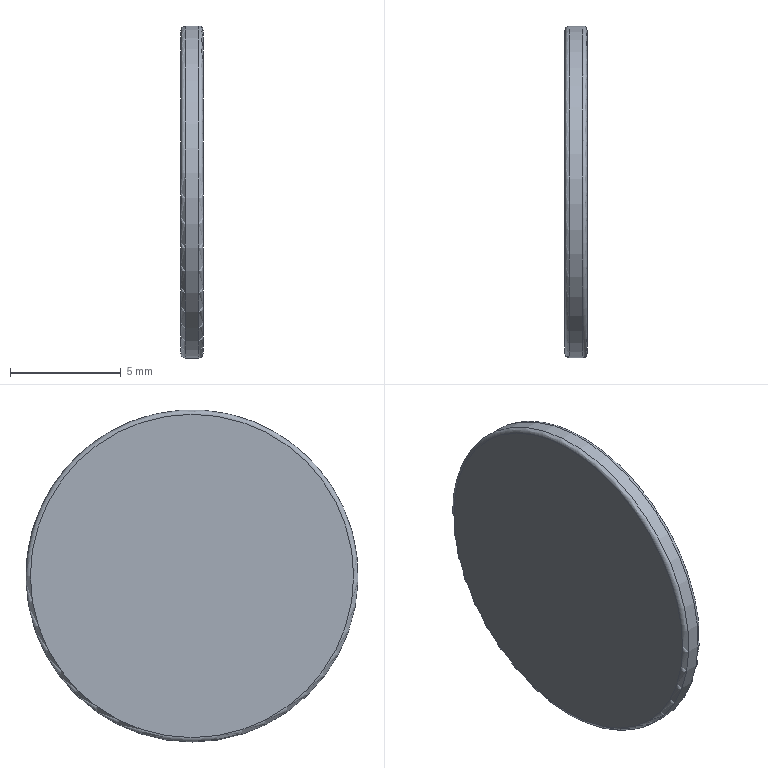Part | STEP file | Tube necking machine_id234_x_t | 1 solid | 5 faces | box 1 x 15 x 15 mm | volume 175.91 mm3 | plane 2 | torus 2 | cylinder 1 | commonest cylinder face diameters 15 x1
STEP:
#1=CARTESIAN_POINT('',(0.,0.,0.));
#2=DIRECTION('',(0.,0.,1.));
#3=DIRECTION('',(1.,0.,0.));
#4=AXIS2_PLACEMENT_3D('',#1,#2,#3);
#5=CARTESIAN_POINT('',(-132.7,-84.,252.5));
#6=VERTEX_POINT('',#5);
#7=CARTESIAN_POINT('',(-132.7,-84.,260.));
#8=DIRECTION('',(-1.,0.,0.));
#9=DIRECTION('',(0.,0.,-1.));
#10=AXIS2_PLACEMENT_3D('',#7,#8,#9);
#11=CIRCLE('',#10,7.5);
#12=CARTESIAN_POINT('',(-133.5,-84.,260.));
#13=DIRECTION('',(1.,0.,0.));
#14=DIRECTION('',(0.,0.,1.));
#15=AXIS2_PLACEMENT_3D('',#12,#13,#14);
#16=CYLINDRICAL_SURFACE('',#15,7.5);
#17=CARTESIAN_POINT('',(9.425,0.8));
#18=DIRECTION('',(-1.,0.));
#19=VECTOR('',#18,1.);
#20=LINE('',#17,#19);
#21=(GEOMETRIC_REPRESENTATION_CONTEXT(2)PARAMETRIC_REPRESENTATION_CONTEXT()REPRESENTATION_CONTEXT('',''));
#22=DEFINITIONAL_REPRESENTATION('',(#20),#21);
#23=PCURVE('',#16,#22);
#24=CARTESIAN_POINT('',(-132.7,-84.,260.));
#25=DIRECTION('',(-1.,0.,0.));
#26=DIRECTION('',(0.,0.,-1.));
#27=AXIS2_PLACEMENT_3D('',#24,#25,#26);
#28=TOROIDAL_SURFACE('',#27,7.3,0.2);
#29=CARTESIAN_POINT('',(0.,6.283));
#30=DIRECTION('',(1.,0.));
#31=VECTOR('',#30,1.);
#32=LINE('',#29,#31);
#33=(GEOMETRIC_REPRESENTATION_CONTEXT(2)PARAMETRIC_REPRESENTATION_CONTEXT()REPRESENTATION_CONTEXT('',''));
#34=DEFINITIONAL_REPRESENTATION('',(#32),#33);
#35=PCURVE('',#28,#34);
#36=SURFACE_CURVE('',#11,(#23,#35),.PCURVE_S1.);
#37=EDGE_CURVE('',#6,#6,#36,.T.);
#38=ORIENTED_EDGE('',*,*,#37,.T.);
#39=CARTESIAN_POINT('',(-133.3,-84.,252.5));
#40=VERTEX_POINT('',#39);
#41=CARTESIAN_POINT('',(-133.3,-84.,252.5));
#42=CARTESIAN_POINT('',(-132.7,-84.,252.5));
#43=B_SPLINE_CURVE_WITH_KNOTS('',1,(#41,#42),.UNSPECIFIED.,.F.,.F.,(2,2),(0.2,0.8),.PIECEWISE_BEZIER_KNOTS.);
#44=CARTESIAN_POINT('',(3.142,0.));
#45=DIRECTION('',(0.,1.));
#46=VECTOR('',#45,1.);
#47=LINE('',#44,#46);
#48=(GEOMETRIC_REPRESENTATION_CONTEXT(2)PARAMETRIC_REPRESENTATION_CONTEXT()REPRESENTATION_CONTEXT('',''));
#49=DEFINITIONAL_REPRESENTATION('',(#47),#48);
#50=PCURVE('',#16,#49);
#51=CARTESIAN_POINT('',(9.425,0.));
#52=DIRECTION('',(0.,1.));
#53=VECTOR('',#52,1.);
#54=LINE('',#51,#53);
#55=(GEOMETRIC_REPRESENTATION_CONTEXT(2)PARAMETRIC_REPRESENTATION_CONTEXT()REPRESENTATION_CONTEXT('',''));
#56=DEFINITIONAL_REPRESENTATION('',(#54),#55);
#57=PCURVE('',#16,#56);
#58=SEAM_CURVE('',#43,(#50,#57),.PCURVE_S1.);
#59=EDGE_CURVE('',#40,#6,#58,.T.);
#60=ORIENTED_EDGE('',*,*,#59,.F.);
#61=CARTESIAN_POINT('',(-133.3,-84.,260.));
#62=DIRECTION('',(1.,0.,0.));
#63=DIRECTION('',(0.,0.,-1.));
#64=AXIS2_PLACEMENT_3D('',#61,#62,#63);
#65=CIRCLE('',#64,7.5);
#66=CARTESIAN_POINT('',(3.142,0.2));
#67=DIRECTION('',(1.,0.));
#68=VECTOR('',#67,1.);
#69=LINE('',#66,#68);
#70=(GEOMETRIC_REPRESENTATION_CONTEXT(2)PARAMETRIC_REPRESENTATION_CONTEXT()REPRESENTATION_CONTEXT('',''));
#71=DEFINITIONAL_REPRESENTATION('',(#69),#70);
#72=PCURVE('',#16,#71);
#73=CARTESIAN_POINT('',(-133.3,-84.,260.));
#74=DIRECTION('',(-1.,0.,0.));
#75=DIRECTION('',(0.,0.,-1.));
#76=AXIS2_PLACEMENT_3D('',#73,#74,#75);
#77=TOROIDAL_SURFACE('',#76,7.3,0.2);
#78=CARTESIAN_POINT('',(6.283,6.283));
#79=DIRECTION('',(-1.,0.));
#80=VECTOR('',#79,1.);
#81=LINE('',#78,#80);
#82=(GEOMETRIC_REPRESENTATION_CONTEXT(2)PARAMETRIC_REPRESENTATION_CONTEXT()REPRESENTATION_CONTEXT('',''));
#83=DEFINITIONAL_REPRESENTATION('',(#81),#82);
#84=PCURVE('',#77,#83);
#85=SURFACE_CURVE('',#65,(#72,#84),.PCURVE_S1.);
#86=EDGE_CURVE('',#40,#40,#85,.T.);
#87=ORIENTED_EDGE('',*,*,#86,.T.);
#88=ORIENTED_EDGE('',*,*,#59,.T.);
#89=EDGE_LOOP('',(#38,#60,#87,#88));
#90=FACE_BOUND('',#89,.T.);
#91=ADVANCED_FACE('',(#90),#16,.T.);
#92=CARTESIAN_POINT('',(-133.5,-84.,252.7));
#93=VERTEX_POINT('',#92);
#94=CARTESIAN_POINT('',(-133.5,-84.,260.));
#95=DIRECTION('',(-1.,0.,0.));
#96=DIRECTION('',(0.,0.,-1.));
#97=AXIS2_PLACEMENT_3D('',#94,#95,#96);
#98=CIRCLE('',#97,7.3);
#99=CARTESIAN_POINT('',(-133.5,-84.,260.));
#100=DIRECTION('',(-1.,0.,0.));
#101=DIRECTION('',(0.,0.,-1.));
#102=AXIS2_PLACEMENT_3D('',#99,#100,#101);
#103=PLANE('',#102);
#104=CARTESIAN_POINT('',(0.,0.));
#105=DIRECTION('',(1.,0.));
#106=AXIS2_PLACEMENT_2D('',#104,#105);
#107=CIRCLE('',#106,7.3);
#108=(GEOMETRIC_REPRESENTATION_CONTEXT(2)PARAMETRIC_REPRESENTATION_CONTEXT()REPRESENTATION_CONTEXT('',''));
#109=DEFINITIONAL_REPRESENTATION('',(#107),#108);
#110=PCURVE('',#103,#109);
#111=CARTESIAN_POINT('',(0.,7.854));
#112=DIRECTION('',(1.,0.));
#113=VECTOR('',#112,1.);
#114=LINE('',#111,#113);
#115=(GEOMETRIC_REPRESENTATION_CONTEXT(2)PARAMETRIC_REPRESENTATION_CONTEXT()REPRESENTATION_CONTEXT('',''));
#116=DEFINITIONAL_REPRESENTATION('',(#114),#115);
#117=PCURVE('',#77,#116);
#118=SURFACE_CURVE('',#98,(#110,#117),.PCURVE_S1.);
#119=EDGE_CURVE('',#93,#93,#118,.T.);
#120=ORIENTED_EDGE('',*,*,#119,.T.);
#121=EDGE_LOOP('',(#120));
#122=FACE_BOUND('',#121,.T.);
#123=ADVANCED_FACE('',(#122),#103,.T.);
#124=CARTESIAN_POINT('',(-132.5,-84.,252.7));
#125=VERTEX_POINT('',#124);
#126=CARTESIAN_POINT('',(-132.5,-84.,260.));
#127=DIRECTION('',(1.,0.,0.));
#128=DIRECTION('',(0.,0.,-1.));
#129=AXIS2_PLACEMENT_3D('',#126,#127,#128);
#130=CIRCLE('',#129,7.3);
#131=CARTESIAN_POINT('',(-132.5,-84.,260.));
#132=DIRECTION('',(-1.,0.,0.));
#133=DIRECTION('',(0.,0.,-1.));
#134=AXIS2_PLACEMENT_3D('',#131,#132,#133);
#135=PLANE('',#134);
#136=CARTESIAN_POINT('',(7.3,0.));
#137=CARTESIAN_POINT('',(7.3,-12.644));
#138=CARTESIAN_POINT('',(-3.65,-6.322));
#139=CARTESIAN_POINT('',(-14.6,0.));
#140=CARTESIAN_POINT('',(-3.65,6.322));
#141=CARTESIAN_POINT('',(7.3,12.644));
#142=CARTESIAN_POINT('',(7.3,0.));
#143=(BOUNDED_CURVE()B_SPLINE_CURVE(2,(#136,#137,#138,#139,#140,#141,#142),.UNSPECIFIED.,.T.,.F.)B_SPLINE_CURVE_WITH_KNOTS((1,2,2,2,2,1),(-2.094,0.,2.094,4.189,6.283,8.378),.UNSPECIFIED.)CURVE()GEOMETRIC_REPRESENTATION_ITEM()RATIONAL_B_SPLINE_CURVE((1.,0.5,1.,0.5,1.,0.5,1.))REPRESENTATION_ITEM(''));
#144=(GEOMETRIC_REPRESENTATION_CONTEXT(2)PARAMETRIC_REPRESENTATION_CONTEXT()REPRESENTATION_CONTEXT('',''));
#145=DEFINITIONAL_REPRESENTATION('',(#143),#144);
#146=PCURVE('',#135,#145);
#147=CARTESIAN_POINT('',(6.283,4.712));
#148=DIRECTION('',(-1.,0.));
#149=VECTOR('',#148,1.);
#150=LINE('',#147,#149);
#151=(GEOMETRIC_REPRESENTATION_CONTEXT(2)PARAMETRIC_REPRESENTATION_CONTEXT()REPRESENTATION_CONTEXT('',''));
#152=DEFINITIONAL_REPRESENTATION('',(#150),#151);
#153=PCURVE('',#28,#152);
#154=SURFACE_CURVE('',#130,(#146,#153),.PCURVE_S1.);
#155=EDGE_CURVE('',#125,#125,#154,.T.);
#156=ORIENTED_EDGE('',*,*,#155,.T.);
#157=EDGE_LOOP('',(#156));
#158=FACE_BOUND('',#157,.T.);
#159=ADVANCED_FACE('',(#158),#135,.F.);
#160=ORIENTED_EDGE('',*,*,#155,.F.);
#161=CARTESIAN_POINT('',(-132.5,-84.,252.7));
#162=CARTESIAN_POINT('',(-132.5,-84.,252.647));
#163=CARTESIAN_POINT('',(-132.517,-84.,252.594));
#164=CARTESIAN_POINT('',(-132.55,-84.,252.55));
#165=CARTESIAN_POINT('',(-132.594,-84.,252.517));
#166=CARTESIAN_POINT('',(-132.647,-84.,252.5));
#167=CARTESIAN_POINT('',(-132.7,-84.,252.5));
#168=(BOUNDED_CURVE()B_SPLINE_CURVE(6,(#161,#162,#163,#164,#165,#166,#167),.UNSPECIFIED.,.F.,.F.)B_SPLINE_CURVE_WITH_KNOTS((7,7),(4.712,6.283),.PIECEWISE_BEZIER_KNOTS.)CURVE()GEOMETRIC_REPRESENTATION_ITEM()RATIONAL_B_SPLINE_CURVE((1.031,1.01,0.9979,0.994,0.9979,1.01,1.031))REPRESENTATION_ITEM(''));
#169=CARTESIAN_POINT('',(6.283,0.));
#170=DIRECTION('',(0.,1.));
#171=VECTOR('',#170,1.);
#172=LINE('',#169,#171);
#173=(GEOMETRIC_REPRESENTATION_CONTEXT(2)PARAMETRIC_REPRESENTATION_CONTEXT()REPRESENTATION_CONTEXT('',''));
#174=DEFINITIONAL_REPRESENTATION('',(#172),#173);
#175=PCURVE('',#28,#174);
#176=CARTESIAN_POINT('',(0.,0.));
#177=DIRECTION('',(0.,1.));
#178=VECTOR('',#177,1.);
#179=LINE('',#176,#178);
#180=(GEOMETRIC_REPRESENTATION_CONTEXT(2)PARAMETRIC_REPRESENTATION_CONTEXT()REPRESENTATION_CONTEXT('',''));
#181=DEFINITIONAL_REPRESENTATION('',(#179),#180);
#182=PCURVE('',#28,#181);
#183=SEAM_CURVE('',#168,(#175,#182),.PCURVE_S1.);
#184=EDGE_CURVE('',#125,#6,#183,.T.);
#185=ORIENTED_EDGE('',*,*,#184,.T.);
#186=ORIENTED_EDGE('',*,*,#37,.F.);
#187=ORIENTED_EDGE('',*,*,#184,.F.);
#188=EDGE_LOOP('',(#160,#185,#186,#187));
#189=FACE_BOUND('',#188,.T.);
#190=ADVANCED_FACE('',(#189),#28,.T.);
#191=ORIENTED_EDGE('',*,*,#86,.F.);
#192=CARTESIAN_POINT('',(-133.3,-84.,252.5));
#193=CARTESIAN_POINT('',(-133.353,-84.,252.5));
#194=CARTESIAN_POINT('',(-133.406,-84.,252.517));
#195=CARTESIAN_POINT('',(-133.45,-84.,252.55));
#196=CARTESIAN_POINT('',(-133.483,-84.,252.594));
#197=CARTESIAN_POINT('',(-133.5,-84.,252.647));
#198=CARTESIAN_POINT('',(-133.5,-84.,252.7));
#199=(BOUNDED_CURVE()B_SPLINE_CURVE(6,(#192,#193,#194,#195,#196,#197,#198),.UNSPECIFIED.,.F.,.F.)B_SPLINE_CURVE_WITH_KNOTS((7,7),(0.,1.571),.PIECEWISE_BEZIER_KNOTS.)CURVE()GEOMETRIC_REPRESENTATION_ITEM()RATIONAL_B_SPLINE_CURVE((1.031,1.01,0.9979,0.994,0.9979,1.01,1.031))REPRESENTATION_ITEM(''));
#200=CARTESIAN_POINT('',(6.283,6.283));
#201=DIRECTION('',(0.,1.));
#202=VECTOR('',#201,1.);
#203=LINE('',#200,#202);
#204=(GEOMETRIC_REPRESENTATION_CONTEXT(2)PARAMETRIC_REPRESENTATION_CONTEXT()REPRESENTATION_CONTEXT('',''));
#205=DEFINITIONAL_REPRESENTATION('',(#203),#204);
#206=PCURVE('',#77,#205);
#207=CARTESIAN_POINT('',(0.,6.283));
#208=DIRECTION('',(0.,1.));
#209=VECTOR('',#208,1.);
#210=LINE('',#207,#209);
#211=(GEOMETRIC_REPRESENTATION_CONTEXT(2)PARAMETRIC_REPRESENTATION_CONTEXT()REPRESENTATION_CONTEXT('',''));
#212=DEFINITIONAL_REPRESENTATION('',(#210),#211);
#213=PCURVE('',#77,#212);
#214=SEAM_CURVE('',#199,(#206,#213),.PCURVE_S1.);
#215=EDGE_CURVE('',#40,#93,#214,.T.);
#216=ORIENTED_EDGE('',*,*,#215,.T.);
#217=ORIENTED_EDGE('',*,*,#119,.F.);
#218=ORIENTED_EDGE('',*,*,#215,.F.);
#219=EDGE_LOOP('',(#191,#216,#217,#218));
#220=FACE_BOUND('',#219,.T.);
#221=ADVANCED_FACE('',(#220),#77,.T.);
#222=CLOSED_SHELL('',(#91,#123,#159,#190,#221));
#223=MANIFOLD_SOLID_BREP('',#222);
#224=(LENGTH_UNIT()NAMED_UNIT(*)SI_UNIT(.MILLI.,.METRE.));
#225=UNCERTAINTY_MEASURE_WITH_UNIT(LENGTH_MEASURE(0.00001),#224,'','');
#226=(NAMED_UNIT(*)PLANE_ANGLE_UNIT()SI_UNIT($,.RADIAN.));
#227=(NAMED_UNIT(*)SI_UNIT($,.STERADIAN.)SOLID_ANGLE_UNIT());
#228=(GEOMETRIC_REPRESENTATION_CONTEXT(3)GLOBAL_UNCERTAINTY_ASSIGNED_CONTEXT((#225))GLOBAL_UNIT_ASSIGNED_CONTEXT((#224,#226,#227))REPRESENTATION_CONTEXT('',''));
#229=ADVANCED_BREP_SHAPE_REPRESENTATION('',(#4,#223),#228);